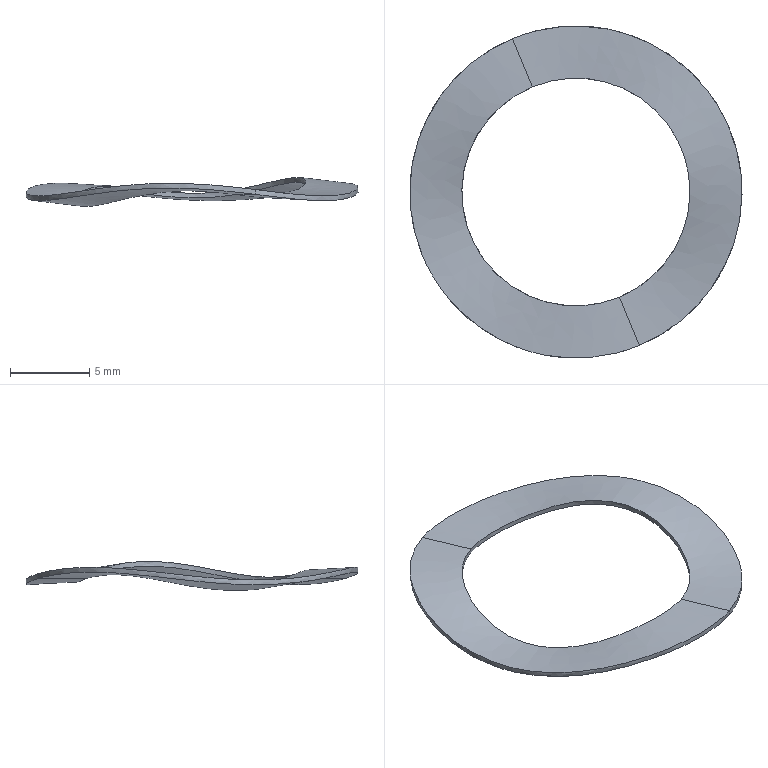Part | STEP file | MSBR-23_1_1_1_1 | 1 solid | 8 faces | box 21.008 x 21.003 x 1.851 mm | volume 55.347 mm3 | spline 4 | other 4
STEP:
#1=CARTESIAN_POINT('',(0.,0.,0.));
#2=DIRECTION('',(0.,0.,1.));
#3=DIRECTION('',(1.,0.,0.));
#4=AXIS2_PLACEMENT_3D('',#1,#2,#3);
#5=CARTESIAN_POINT('',(4.014,-9.702,86.503));
#6=VERTEX_POINT('',#5);
#7=CARTESIAN_POINT('',(2.75,-6.654,86.503));
#8=VERTEX_POINT('',#7);
#9=CARTESIAN_POINT('',(4.014,-9.702,86.503));
#10=DIRECTION('',(-0.383,0.9237,0.));
#11=VECTOR('',#10,3.3);
#12=LINE('',#9,#11);
#13=EDGE_CURVE('',#6,#8,#12,.T.);
#14=ORIENTED_EDGE('',*,*,#13,.F.);
#15=CARTESIAN_POINT('',(-4.03,9.696,86.503));
#16=VERTEX_POINT('',#15);
#17=CARTESIAN_POINT('',(-4.466,9.515,86.557));
#18=CARTESIAN_POINT('',(-5.302,9.099,86.663));
#19=CARTESIAN_POINT('',(-6.432,8.338,86.794));
#20=CARTESIAN_POINT('',(-7.446,7.45,86.881));
#21=CARTESIAN_POINT('',(-8.359,6.409,86.913));
#22=CARTESIAN_POINT('',(-9.107,5.296,86.884));
#23=CARTESIAN_POINT('',(-9.73,4.041,86.795));
#24=CARTESIAN_POINT('',(-10.168,2.76,86.665));
#25=CARTESIAN_POINT('',(-10.445,1.402,86.507));
#26=CARTESIAN_POINT('',(-10.54,-0.01496,86.345));
#27=CARTESIAN_POINT('',(-10.442,-1.421,86.209));
#28=CARTESIAN_POINT('',(-10.167,-2.768,86.122));
#29=CARTESIAN_POINT('',(-9.732,-4.039,86.093));
#30=CARTESIAN_POINT('',(-9.127,-5.267,86.124));
#31=CARTESIAN_POINT('',(-8.371,-6.401,86.211));
#32=CARTESIAN_POINT('',(-7.449,-7.456,86.346));
#33=CARTESIAN_POINT('',(-6.386,-8.382,86.507));
#34=CARTESIAN_POINT('',(-5.241,-9.14,86.663));
#35=CARTESIAN_POINT('',(-4.007,-9.746,86.796));
#36=CARTESIAN_POINT('',(-2.671,-10.19,86.884));
#37=CARTESIAN_POINT('',(-1.362,-10.445,86.913));
#38=CARTESIAN_POINT('',(0.02789,-10.533,86.88));
#39=CARTESIAN_POINT('',(1.365,-10.441,86.793));
#40=CARTESIAN_POINT('',(2.695,-10.18,86.663));
#41=CARTESIAN_POINT('',(3.579,-9.883,86.557));
#42=CARTESIAN_POINT('',(4.014,-9.702,86.503));
#43=B_SPLINE_CURVE_WITH_KNOTS('',3,(#15,#17,#18,#19,#20,#21,#22,#23,#24,#25,#26,#27,#28,#29,#30,#31,#32,#33,#34,#35,#36,#37,#38,#39,#40,#41,#42),.UNSPECIFIED.,.F.,.F.,(4,1,1,1,1,1,1,1,1,1,1,1,1,1,1,1,1,1,1,1,1,1,1,1,4),(0.,0.04167,0.08333,0.125,0.1667,0.2083,0.25,0.2917,0.3333,0.375,0.4167,0.4583,0.5,0.5417,0.5833,0.625,0.6667,0.7083,0.75,0.7917,0.8333,0.875,0.9167,0.9583,1.),.UNSPECIFIED.);
#44=EDGE_CURVE('',#16,#6,#43,.T.);
#45=ORIENTED_EDGE('',*,*,#44,.F.);
#46=CARTESIAN_POINT('',(-2.766,6.648,86.503));
#47=VERTEX_POINT('',#46);
#48=CARTESIAN_POINT('',(-2.766,6.648,86.503));
#49=DIRECTION('',(-0.383,0.9237,0.));
#50=VECTOR('',#49,3.3);
#51=LINE('',#48,#50);
#52=EDGE_CURVE('',#47,#16,#51,.T.);
#53=ORIENTED_EDGE('',*,*,#52,.F.);
#54=CARTESIAN_POINT('',(2.75,-6.654,86.503));
#55=CARTESIAN_POINT('',(2.431,-6.787,86.542));
#56=CARTESIAN_POINT('',(1.789,-6.999,86.618));
#57=CARTESIAN_POINT('',(0.8599,-7.171,86.699));
#58=CARTESIAN_POINT('',(-0.05536,-7.228,86.74));
#59=CARTESIAN_POINT('',(-1.07,-7.152,86.717));
#60=CARTESIAN_POINT('',(-1.966,-6.963,86.639));
#61=CARTESIAN_POINT('',(-2.947,-6.616,86.492));
#62=CARTESIAN_POINT('',(-3.833,-6.146,86.306));
#63=CARTESIAN_POINT('',(-4.631,-5.575,86.112));
#64=CARTESIAN_POINT('',(-5.371,-4.874,85.931));
#65=CARTESIAN_POINT('',(-6.022,-4.041,85.793));
#66=CARTESIAN_POINT('',(-6.494,-3.221,85.726));
#67=CARTESIAN_POINT('',(-6.856,-2.357,85.725));
#68=CARTESIAN_POINT('',(-7.111,-1.427,85.791));
#69=CARTESIAN_POINT('',(-7.241,-0.395,85.925));
#70=CARTESIAN_POINT('',(-7.222,0.593,86.099));
#71=CARTESIAN_POINT('',(-7.076,1.556,86.291));
#72=CARTESIAN_POINT('',(-6.782,2.546,86.484));
#73=CARTESIAN_POINT('',(-6.339,3.488,86.634));
#74=CARTESIAN_POINT('',(-5.834,4.274,86.715));
#75=CARTESIAN_POINT('',(-5.171,5.053,86.74));
#76=CARTESIAN_POINT('',(-4.467,5.677,86.7));
#77=CARTESIAN_POINT('',(-3.685,6.213,86.618));
#78=CARTESIAN_POINT('',(-3.083,6.516,86.542));
#79=CARTESIAN_POINT('',(-2.766,6.648,86.503));
#80=B_SPLINE_CURVE_WITH_KNOTS('',3,(#54,#55,#56,#57,#58,#59,#60,#61,#62,#63,#64,#65,#66,#67,#68,#69,#70,#71,#72,#73,#74,#75,#76,#77,#78,#79),.UNSPECIFIED.,.F.,.F.,(4,1,1,1,1,1,1,1,1,1,1,1,1,1,1,1,1,1,1,1,1,1,1,4),(0.,0.04348,0.08696,0.1304,0.1739,0.2174,0.2609,0.3043,0.3478,0.3913,0.4348,0.4783,0.5217,0.5652,0.6087,0.6522,0.6957,0.7391,0.7826,0.8261,0.8696,0.913,0.9565,1.),.UNSPECIFIED.);
#81=EDGE_CURVE('',#8,#47,#80,.T.);
#82=ORIENTED_EDGE('',*,*,#81,.F.);
#83=EDGE_LOOP('',(#14,#45,#53,#82));
#84=FACE_OUTER_BOUND('',#83,.F.);
#85=CARTESIAN_POINT('',(4.643,-9.491,86.428));
#86=CARTESIAN_POINT('',(4.14,-8.463,86.436));
#87=CARTESIAN_POINT('',(3.637,-7.436,86.444));
#88=CARTESIAN_POINT('',(3.135,-6.408,86.452));
#89=CARTESIAN_POINT('',(4.445,-9.588,86.452));
#90=CARTESIAN_POINT('',(3.963,-8.55,86.458));
#91=CARTESIAN_POINT('',(3.482,-7.512,86.463));
#92=CARTESIAN_POINT('',(3.,-6.474,86.469));
#93=CARTESIAN_POINT('',(3.805,-9.877,86.533));
#94=CARTESIAN_POINT('',(3.392,-8.808,86.529));
#95=CARTESIAN_POINT('',(2.979,-7.739,86.526));
#96=CARTESIAN_POINT('',(2.566,-6.67,86.523));
#97=CARTESIAN_POINT('',(2.682,-10.255,86.668));
#98=CARTESIAN_POINT('',(2.388,-9.146,86.65));
#99=CARTESIAN_POINT('',(2.095,-8.037,86.632));
#100=CARTESIAN_POINT('',(1.802,-6.927,86.615));
#101=CARTESIAN_POINT('',(1.261,-10.526,86.805));
#102=CARTESIAN_POINT('',(1.12,-9.387,86.77));
#103=CARTESIAN_POINT('',(0.9801,-8.249,86.735));
#104=CARTESIAN_POINT('',(0.8399,-7.111,86.7));
#105=CARTESIAN_POINT('',(-0.1842,-10.601,86.893));
#106=CARTESIAN_POINT('',(-0.1673,-9.454,86.841));
#107=CARTESIAN_POINT('',(-0.1505,-8.308,86.789));
#108=CARTESIAN_POINT('',(-0.1336,-7.161,86.738));
#109=CARTESIAN_POINT('',(-1.626,-10.478,86.917));
#110=CARTESIAN_POINT('',(-1.45,-9.345,86.849));
#111=CARTESIAN_POINT('',(-1.275,-8.213,86.781));
#112=CARTESIAN_POINT('',(-1.1,-7.081,86.713));
#113=CARTESIAN_POINT('',(-3.037,-10.16,86.873));
#114=CARTESIAN_POINT('',(-2.706,-9.064,86.79));
#115=CARTESIAN_POINT('',(-2.374,-7.968,86.707));
#116=CARTESIAN_POINT('',(-2.043,-6.872,86.624));
#117=CARTESIAN_POINT('',(-4.392,-9.652,86.768));
#118=CARTESIAN_POINT('',(-3.911,-8.615,86.672));
#119=CARTESIAN_POINT('',(-3.43,-7.577,86.576));
#120=CARTESIAN_POINT('',(-2.949,-6.539,86.479));
#121=CARTESIAN_POINT('',(-5.665,-8.965,86.62));
#122=CARTESIAN_POINT('',(-5.045,-8.006,86.513));
#123=CARTESIAN_POINT('',(-4.425,-7.046,86.405));
#124=CARTESIAN_POINT('',(-3.805,-6.086,86.298));
#125=CARTESIAN_POINT('',(-6.833,-8.111,86.454));
#126=CARTESIAN_POINT('',(-6.087,-7.247,86.337));
#127=CARTESIAN_POINT('',(-5.342,-6.382,86.22));
#128=CARTESIAN_POINT('',(-4.596,-5.518,86.104));
#129=CARTESIAN_POINT('',(-7.873,-7.106,86.296));
#130=CARTESIAN_POINT('',(-7.018,-6.351,86.173));
#131=CARTESIAN_POINT('',(-6.164,-5.596,86.05));
#132=CARTESIAN_POINT('',(-5.309,-4.841,85.926));
#133=CARTESIAN_POINT('',(-8.767,-5.969,86.174));
#134=CARTESIAN_POINT('',(-7.82,-5.335,86.046));
#135=CARTESIAN_POINT('',(-6.873,-4.7,85.919));
#136=CARTESIAN_POINT('',(-5.926,-4.065,85.791));
#137=CARTESIAN_POINT('',(-9.498,-4.721,86.108));
#138=CARTESIAN_POINT('',(-8.476,-4.217,85.978));
#139=CARTESIAN_POINT('',(-7.454,-3.712,85.848));
#140=CARTESIAN_POINT('',(-6.432,-3.207,85.718));
#141=CARTESIAN_POINT('',(-10.052,-3.385,86.108));
#142=CARTESIAN_POINT('',(-8.973,-3.019,85.978));
#143=CARTESIAN_POINT('',(-7.893,-2.652,85.848));
#144=CARTESIAN_POINT('',(-6.814,-2.285,85.718));
#145=CARTESIAN_POINT('',(-10.419,-1.987,86.174));
#146=CARTESIAN_POINT('',(-9.3,-1.765,86.046));
#147=CARTESIAN_POINT('',(-8.182,-1.543,85.919));
#148=CARTESIAN_POINT('',(-7.064,-1.321,85.791));
#149=CARTESIAN_POINT('',(-10.592,-0.5507,86.296));
#150=CARTESIAN_POINT('',(-9.453,-0.4793,86.173));
#151=CARTESIAN_POINT('',(-8.315,-0.408,86.05));
#152=CARTESIAN_POINT('',(-7.176,-0.3367,85.926));
#153=CARTESIAN_POINT('',(-10.568,0.8956,86.454));
#154=CARTESIAN_POINT('',(-9.429,0.8123,86.337));
#155=CARTESIAN_POINT('',(-8.291,0.7291,86.22));
#156=CARTESIAN_POINT('',(-7.152,0.6458,86.104));
#157=CARTESIAN_POINT('',(-10.347,2.325,86.62));
#158=CARTESIAN_POINT('',(-9.23,2.086,86.513));
#159=CARTESIAN_POINT('',(-8.113,1.847,86.405));
#160=CARTESIAN_POINT('',(-6.995,1.608,86.298));
#161=CARTESIAN_POINT('',(-9.934,3.712,86.768));
#162=CARTESIAN_POINT('',(-8.86,3.319,86.672));
#163=CARTESIAN_POINT('',(-7.786,2.926,86.576));
#164=CARTESIAN_POINT('',(-6.711,2.534,86.479));
#165=CARTESIAN_POINT('',(-9.336,5.029,86.873));
#166=CARTESIAN_POINT('',(-8.326,4.489,86.79));
#167=CARTESIAN_POINT('',(-7.316,3.95,86.707));
#168=CARTESIAN_POINT('',(-6.307,3.41,86.624));
#169=CARTESIAN_POINT('',(-8.563,6.253,86.917));
#170=CARTESIAN_POINT('',(-7.638,5.577,86.849));
#171=CARTESIAN_POINT('',(-6.713,4.901,86.781));
#172=CARTESIAN_POINT('',(-5.788,4.225,86.713));
#173=CARTESIAN_POINT('',(-7.632,7.359,86.893));
#174=CARTESIAN_POINT('',(-6.809,6.561,86.841));
#175=CARTESIAN_POINT('',(-5.985,5.763,86.789));
#176=CARTESIAN_POINT('',(-5.162,4.965,86.738));
#177=CARTESIAN_POINT('',(-6.558,8.329,86.805));
#178=CARTESIAN_POINT('',(-5.852,7.425,86.77));
#179=CARTESIAN_POINT('',(-5.145,6.522,86.735));
#180=CARTESIAN_POINT('',(-4.438,5.618,86.7));
#181=CARTESIAN_POINT('',(-5.363,9.143,86.668));
#182=CARTESIAN_POINT('',(-4.785,8.152,86.65));
#183=CARTESIAN_POINT('',(-4.207,7.161,86.632));
#184=CARTESIAN_POINT('',(-3.629,6.17,86.615));
#185=CARTESIAN_POINT('',(-4.301,9.671,86.533));
#186=CARTESIAN_POINT('',(-3.837,8.624,86.529));
#187=CARTESIAN_POINT('',(-3.372,7.576,86.526));
#188=CARTESIAN_POINT('',(-2.908,6.528,86.523));
#189=CARTESIAN_POINT('',(-3.645,9.92,86.452));
#190=CARTESIAN_POINT('',(-3.25,8.845,86.458));
#191=CARTESIAN_POINT('',(-2.856,7.771,86.463));
#192=CARTESIAN_POINT('',(-2.462,6.697,86.469));
#193=CARTESIAN_POINT('',(-3.436,9.991,86.428));
#194=CARTESIAN_POINT('',(-3.064,8.909,86.436));
#195=CARTESIAN_POINT('',(-2.692,7.828,86.444));
#196=CARTESIAN_POINT('',(-2.32,6.746,86.452));
#197=B_SPLINE_SURFACE_WITH_KNOTS('',3,3,((#85,#86,#87,#88),(#89,#90,#91,#92),(#93,#94,#95,#96),(#97,#98,#99,#100),(#101,#102,#103,#104),(#105,#106,#107,#108),(#109,#110,#111,#112),(#113,#114,#115,#116),(#117,#118,#119,#120),(#121,#122,#123,#124),(#125,#126,#127,#128),(#129,#130,#131,#132),(#133,#134,#135,#136),(#137,#138,#139,#140),(#141,#142,#143,#144),(#145,#146,#147,#148),(#149,#150,#151,#152),(#153,#154,#155,#156),(#157,#158,#159,#160),(#161,#162,#163,#164),(#165,#166,#167,#168),(#169,#170,#171,#172),(#173,#174,#175,#176),(#177,#178,#179,#180),(#181,#182,#183,#184),(#185,#186,#187,#188),(#189,#190,#191,#192),(#193,#194,#195,#196)),.UNSPECIFIED.,.F.,.F.,.F.,(4,1,1,1,1,1,1,1,1,1,1,1,1,1,1,1,1,1,1,1,1,1,1,1,1,4),(4,4),(-0.01993,0.,0.04348,0.08696,0.1304,0.1739,0.2174,0.2609,0.3043,0.3478,0.3913,0.4348,0.4783,0.5217,0.5652,0.6087,0.6522,0.6957,0.7391,0.7826,0.8261,0.8696,0.913,0.9565,1.,1.02),(-0.000000563,1.),.UNSPECIFIED.);
#198=ADVANCED_FACE('',(#84),#197,.F.);
#199=CARTESIAN_POINT('',(-2.766,6.648,86.503));
#200=CARTESIAN_POINT('',(-2.446,6.78,86.463));
#201=CARTESIAN_POINT('',(-1.804,6.992,86.388));
#202=CARTESIAN_POINT('',(-0.875,7.165,86.306));
#203=CARTESIAN_POINT('',(0.04021,7.222,86.266));
#204=CARTESIAN_POINT('',(1.055,7.145,86.289));
#205=CARTESIAN_POINT('',(1.951,6.956,86.367));
#206=CARTESIAN_POINT('',(2.932,6.61,86.514));
#207=CARTESIAN_POINT('',(3.818,6.14,86.699));
#208=CARTESIAN_POINT('',(4.616,5.569,86.893));
#209=CARTESIAN_POINT('',(5.356,4.868,87.075));
#210=CARTESIAN_POINT('',(6.007,4.035,87.213));
#211=CARTESIAN_POINT('',(6.479,3.215,87.279));
#212=CARTESIAN_POINT('',(6.841,2.351,87.28));
#213=CARTESIAN_POINT('',(7.096,1.421,87.214));
#214=CARTESIAN_POINT('',(7.226,0.3888,87.08));
#215=CARTESIAN_POINT('',(7.207,-0.5992,86.907));
#216=CARTESIAN_POINT('',(7.061,-1.562,86.714));
#217=CARTESIAN_POINT('',(6.767,-2.552,86.522));
#218=CARTESIAN_POINT('',(6.324,-3.495,86.372));
#219=CARTESIAN_POINT('',(5.819,-4.28,86.29));
#220=CARTESIAN_POINT('',(5.155,-5.059,86.265));
#221=CARTESIAN_POINT('',(4.452,-5.683,86.306));
#222=CARTESIAN_POINT('',(3.67,-6.219,86.388));
#223=CARTESIAN_POINT('',(3.068,-6.522,86.464));
#224=CARTESIAN_POINT('',(2.75,-6.654,86.503));
#225=B_SPLINE_CURVE_WITH_KNOTS('',3,(#199,#200,#201,#202,#203,#204,#205,#206,#207,#208,#209,#210,#211,#212,#213,#214,#215,#216,#217,#218,#219,#220,#221,#222,#223,#224),.UNSPECIFIED.,.F.,.F.,(4,1,1,1,1,1,1,1,1,1,1,1,1,1,1,1,1,1,1,1,1,1,1,4),(0.,0.04348,0.08696,0.1304,0.1739,0.2174,0.2609,0.3043,0.3478,0.3913,0.4348,0.4783,0.5217,0.5652,0.6087,0.6522,0.6957,0.7391,0.7826,0.8261,0.8696,0.913,0.9565,1.),.UNSPECIFIED.);
#226=EDGE_CURVE('',#47,#8,#225,.T.);
#227=ORIENTED_EDGE('',*,*,#226,.F.);
#228=ORIENTED_EDGE('',*,*,#52,.T.);
#229=CARTESIAN_POINT('',(4.014,-9.702,86.503));
#230=CARTESIAN_POINT('',(4.448,-9.523,86.449));
#231=CARTESIAN_POINT('',(5.28,-9.109,86.345));
#232=CARTESIAN_POINT('',(6.406,-8.352,86.214));
#233=CARTESIAN_POINT('',(7.42,-7.467,86.124));
#234=CARTESIAN_POINT('',(8.335,-6.426,86.096));
#235=CARTESIAN_POINT('',(9.083,-5.317,86.124));
#236=CARTESIAN_POINT('',(9.712,-4.057,86.21));
#237=CARTESIAN_POINT('',(10.15,-2.776,86.34));
#238=CARTESIAN_POINT('',(10.428,-1.421,86.498));
#239=CARTESIAN_POINT('',(10.525,-0.00639,86.659));
#240=CARTESIAN_POINT('',(10.428,1.411,86.794));
#241=CARTESIAN_POINT('',(10.151,2.764,86.882));
#242=CARTESIAN_POINT('',(9.719,4.027,86.913));
#243=CARTESIAN_POINT('',(9.114,5.257,86.881));
#244=CARTESIAN_POINT('',(8.36,6.39,86.793));
#245=CARTESIAN_POINT('',(7.434,7.449,86.66));
#246=CARTESIAN_POINT('',(6.371,8.376,86.499));
#247=CARTESIAN_POINT('',(5.227,9.133,86.343));
#248=CARTESIAN_POINT('',(3.994,9.738,86.21));
#249=CARTESIAN_POINT('',(2.653,10.185,86.123));
#250=CARTESIAN_POINT('',(1.338,10.44,86.095));
#251=CARTESIAN_POINT('',(-0.0515,10.527,86.125));
#252=CARTESIAN_POINT('',(-1.392,10.434,86.215));
#253=CARTESIAN_POINT('',(-2.716,10.172,86.345));
#254=CARTESIAN_POINT('',(-3.596,9.876,86.449));
#255=CARTESIAN_POINT('',(-4.03,9.696,86.503));
#256=B_SPLINE_CURVE_WITH_KNOTS('',3,(#229,#230,#231,#232,#233,#234,#235,#236,#237,#238,#239,#240,#241,#242,#243,#244,#245,#246,#247,#248,#249,#250,#251,#252,#253,#254,#255),.UNSPECIFIED.,.F.,.F.,(4,1,1,1,1,1,1,1,1,1,1,1,1,1,1,1,1,1,1,1,1,1,1,1,4),(0.,0.04167,0.08333,0.125,0.1667,0.2083,0.25,0.2917,0.3333,0.375,0.4167,0.4583,0.5,0.5417,0.5833,0.625,0.6667,0.7083,0.75,0.7917,0.8333,0.875,0.9167,0.9583,1.),.UNSPECIFIED.);
#257=EDGE_CURVE('',#6,#16,#256,.T.);
#258=ORIENTED_EDGE('',*,*,#257,.F.);
#259=ORIENTED_EDGE('',*,*,#13,.T.);
#260=EDGE_LOOP('',(#227,#228,#258,#259));
#261=FACE_OUTER_BOUND('',#260,.F.);
#262=CARTESIAN_POINT('',(-4.658,9.485,86.578));
#263=CARTESIAN_POINT('',(-4.155,8.457,86.57));
#264=CARTESIAN_POINT('',(-3.652,7.429,86.562));
#265=CARTESIAN_POINT('',(-3.15,6.402,86.554));
#266=CARTESIAN_POINT('',(-4.46,9.582,86.553));
#267=CARTESIAN_POINT('',(-3.978,8.544,86.548));
#268=CARTESIAN_POINT('',(-3.497,7.506,86.542));
#269=CARTESIAN_POINT('',(-3.015,6.468,86.537));
#270=CARTESIAN_POINT('',(-3.82,9.871,86.473));
#271=CARTESIAN_POINT('',(-3.407,8.802,86.476));
#272=CARTESIAN_POINT('',(-2.994,7.733,86.479));
#273=CARTESIAN_POINT('',(-2.581,6.664,86.483));
#274=CARTESIAN_POINT('',(-2.697,10.249,86.338));
#275=CARTESIAN_POINT('',(-2.404,9.14,86.356));
#276=CARTESIAN_POINT('',(-2.111,8.03,86.373));
#277=CARTESIAN_POINT('',(-1.817,6.921,86.391));
#278=CARTESIAN_POINT('',(-1.276,10.52,86.2));
#279=CARTESIAN_POINT('',(-1.135,9.381,86.235));
#280=CARTESIAN_POINT('',(-0.9952,8.243,86.27));
#281=CARTESIAN_POINT('',(-0.855,7.104,86.305));
#282=CARTESIAN_POINT('',(0.1691,10.594,86.112));
#283=CARTESIAN_POINT('',(0.1522,9.448,86.164));
#284=CARTESIAN_POINT('',(0.1354,8.301,86.216));
#285=CARTESIAN_POINT('',(0.1185,7.155,86.268));
#286=CARTESIAN_POINT('',(1.611,10.471,86.088));
#287=CARTESIAN_POINT('',(1.435,9.339,86.157));
#288=CARTESIAN_POINT('',(1.26,8.207,86.225));
#289=CARTESIAN_POINT('',(1.085,7.075,86.293));
#290=CARTESIAN_POINT('',(3.022,10.153,86.133));
#291=CARTESIAN_POINT('',(2.691,9.058,86.216));
#292=CARTESIAN_POINT('',(2.359,7.962,86.299));
#293=CARTESIAN_POINT('',(2.028,6.866,86.382));
#294=CARTESIAN_POINT('',(4.377,9.646,86.238));
#295=CARTESIAN_POINT('',(3.896,8.608,86.334));
#296=CARTESIAN_POINT('',(3.415,7.571,86.43));
#297=CARTESIAN_POINT('',(2.934,6.533,86.526));
#298=CARTESIAN_POINT('',(5.65,8.959,86.386));
#299=CARTESIAN_POINT('',(5.03,7.999,86.493));
#300=CARTESIAN_POINT('',(4.41,7.04,86.601));
#301=CARTESIAN_POINT('',(3.79,6.08,86.708));
#302=CARTESIAN_POINT('',(6.818,8.105,86.552));
#303=CARTESIAN_POINT('',(6.072,7.241,86.669));
#304=CARTESIAN_POINT('',(5.327,6.376,86.785));
#305=CARTESIAN_POINT('',(4.581,5.511,86.902));
#306=CARTESIAN_POINT('',(7.858,7.1,86.709));
#307=CARTESIAN_POINT('',(7.003,6.345,86.833));
#308=CARTESIAN_POINT('',(6.148,5.59,86.956));
#309=CARTESIAN_POINT('',(5.294,4.834,87.079));
#310=CARTESIAN_POINT('',(8.752,5.963,86.832));
#311=CARTESIAN_POINT('',(7.805,5.328,86.959));
#312=CARTESIAN_POINT('',(6.858,4.694,87.087));
#313=CARTESIAN_POINT('',(5.91,4.059,87.215));
#314=CARTESIAN_POINT('',(9.483,4.715,86.898));
#315=CARTESIAN_POINT('',(8.461,4.21,87.028));
#316=CARTESIAN_POINT('',(7.439,3.706,87.158));
#317=CARTESIAN_POINT('',(6.417,3.201,87.288));
#318=CARTESIAN_POINT('',(10.037,3.379,86.898));
#319=CARTESIAN_POINT('',(8.957,3.012,87.028));
#320=CARTESIAN_POINT('',(7.878,2.646,87.158));
#321=CARTESIAN_POINT('',(6.799,2.279,87.288));
#322=CARTESIAN_POINT('',(10.404,1.98,86.832));
#323=CARTESIAN_POINT('',(9.285,1.758,86.959));
#324=CARTESIAN_POINT('',(8.167,1.537,87.087));
#325=CARTESIAN_POINT('',(7.049,1.315,87.215));
#326=CARTESIAN_POINT('',(10.577,0.5444,86.709));
#327=CARTESIAN_POINT('',(9.438,0.4731,86.833));
#328=CARTESIAN_POINT('',(8.3,0.4017,86.956));
#329=CARTESIAN_POINT('',(7.161,0.3304,87.079));
#330=CARTESIAN_POINT('',(10.553,-0.9019,86.552));
#331=CARTESIAN_POINT('',(9.414,-0.8186,86.669));
#332=CARTESIAN_POINT('',(8.276,-0.7353,86.785));
#333=CARTESIAN_POINT('',(7.137,-0.6521,86.902));
#334=CARTESIAN_POINT('',(10.332,-2.332,86.386));
#335=CARTESIAN_POINT('',(9.215,-2.092,86.493));
#336=CARTESIAN_POINT('',(8.098,-1.853,86.601));
#337=CARTESIAN_POINT('',(6.98,-1.614,86.708));
#338=CARTESIAN_POINT('',(9.919,-3.718,86.238));
#339=CARTESIAN_POINT('',(8.845,-3.325,86.334));
#340=CARTESIAN_POINT('',(7.77,-2.933,86.43));
#341=CARTESIAN_POINT('',(6.696,-2.54,86.526));
#342=CARTESIAN_POINT('',(9.32,-5.035,86.133));
#343=CARTESIAN_POINT('',(8.311,-4.496,86.216));
#344=CARTESIAN_POINT('',(7.301,-3.956,86.299));
#345=CARTESIAN_POINT('',(6.292,-3.416,86.382));
#346=CARTESIAN_POINT('',(8.548,-6.259,86.088));
#347=CARTESIAN_POINT('',(7.623,-5.583,86.157));
#348=CARTESIAN_POINT('',(6.698,-4.907,86.225));
#349=CARTESIAN_POINT('',(5.773,-4.231,86.293));
#350=CARTESIAN_POINT('',(7.617,-7.366,86.112));
#351=CARTESIAN_POINT('',(6.793,-6.568,86.164));
#352=CARTESIAN_POINT('',(5.97,-5.77,86.216));
#353=CARTESIAN_POINT('',(5.147,-4.972,86.268));
#354=CARTESIAN_POINT('',(6.543,-8.335,86.2));
#355=CARTESIAN_POINT('',(5.836,-7.432,86.235));
#356=CARTESIAN_POINT('',(5.13,-6.528,86.27));
#357=CARTESIAN_POINT('',(4.423,-5.625,86.305));
#358=CARTESIAN_POINT('',(5.348,-9.15,86.338));
#359=CARTESIAN_POINT('',(4.77,-8.158,86.356));
#360=CARTESIAN_POINT('',(4.192,-7.167,86.373));
#361=CARTESIAN_POINT('',(3.614,-6.176,86.391));
#362=CARTESIAN_POINT('',(4.286,-9.677,86.473));
#363=CARTESIAN_POINT('',(3.822,-8.63,86.476));
#364=CARTESIAN_POINT('',(3.357,-7.582,86.479));
#365=CARTESIAN_POINT('',(2.893,-6.535,86.483));
#366=CARTESIAN_POINT('',(3.63,-9.926,86.553));
#367=CARTESIAN_POINT('',(3.235,-8.852,86.548));
#368=CARTESIAN_POINT('',(2.841,-7.778,86.542));
#369=CARTESIAN_POINT('',(2.447,-6.703,86.537));
#370=CARTESIAN_POINT('',(3.421,-9.997,86.578));
#371=CARTESIAN_POINT('',(3.049,-8.916,86.57));
#372=CARTESIAN_POINT('',(2.677,-7.834,86.562));
#373=CARTESIAN_POINT('',(2.305,-6.752,86.554));
#374=B_SPLINE_SURFACE_WITH_KNOTS('',3,3,((#262,#263,#264,#265),(#266,#267,#268,#269),(#270,#271,#272,#273),(#274,#275,#276,#277),(#278,#279,#280,#281),(#282,#283,#284,#285),(#286,#287,#288,#289),(#290,#291,#292,#293),(#294,#295,#296,#297),(#298,#299,#300,#301),(#302,#303,#304,#305),(#306,#307,#308,#309),(#310,#311,#312,#313),(#314,#315,#316,#317),(#318,#319,#320,#321),(#322,#323,#324,#325),(#326,#327,#328,#329),(#330,#331,#332,#333),(#334,#335,#336,#337),(#338,#339,#340,#341),(#342,#343,#344,#345),(#346,#347,#348,#349),(#350,#351,#352,#353),(#354,#355,#356,#357),(#358,#359,#360,#361),(#362,#363,#364,#365),(#366,#367,#368,#369),(#370,#371,#372,#373)),.UNSPECIFIED.,.F.,.F.,.F.,(4,1,1,1,1,1,1,1,1,1,1,1,1,1,1,1,1,1,1,1,1,1,1,1,1,4),(4,4),(-0.01993,0.,0.04348,0.08696,0.1304,0.1739,0.2174,0.2609,0.3043,0.3478,0.3913,0.4348,0.4783,0.5217,0.5652,0.6087,0.6522,0.6957,0.7391,0.7826,0.8261,0.8696,0.913,0.9565,1.,1.02),(-0.000000504,1.),.UNSPECIFIED.);
#375=ADVANCED_FACE('',(#261),#374,.F.);
#376=CARTESIAN_POINT('',(2.758,-6.651,86.2));
#377=VERTEX_POINT('',#376);
#378=CARTESIAN_POINT('',(2.758,-6.651,86.2));
#379=DIRECTION('',(-0.02492,-0.01034,0.9996));
#380=VECTOR('',#379,0.3029);
#381=LINE('',#378,#380);
#382=EDGE_CURVE('',#377,#8,#381,.T.);
#383=ORIENTED_EDGE('',*,*,#382,.F.);
#384=CARTESIAN_POINT('',(-2.758,6.651,86.2));
#385=VERTEX_POINT('',#384);
#386=CARTESIAN_POINT('',(2.758,-6.651,86.2));
#387=CARTESIAN_POINT('',(3.078,-6.518,86.16));
#388=CARTESIAN_POINT('',(3.681,-6.214,86.085));
#389=CARTESIAN_POINT('',(4.458,-5.68,86.003));
#390=CARTESIAN_POINT('',(5.147,-5.071,85.963));
#391=CARTESIAN_POINT('',(5.808,-4.3,85.986));
#392=CARTESIAN_POINT('',(6.308,-3.532,86.064));
#393=CARTESIAN_POINT('',(6.756,-2.593,86.211));
#394=CARTESIAN_POINT('',(7.05,-1.634,86.397));
#395=CARTESIAN_POINT('',(7.209,-0.6651,86.591));
#396=CARTESIAN_POINT('',(7.237,0.3536,86.772));
#397=CARTESIAN_POINT('',(7.107,1.402,86.909));
#398=CARTESIAN_POINT('',(6.86,2.318,86.976));
#399=CARTESIAN_POINT('',(6.504,3.184,86.978));
#400=CARTESIAN_POINT('',(6.027,4.02,86.912));
#401=CARTESIAN_POINT('',(5.388,4.841,86.778));
#402=CARTESIAN_POINT('',(4.675,5.527,86.604));
#403=CARTESIAN_POINT('',(3.89,6.103,86.412));
#404=CARTESIAN_POINT('',(2.983,6.594,86.219));
#405=CARTESIAN_POINT('',(2.004,6.947,86.069));
#406=CARTESIAN_POINT('',(1.091,7.145,85.987));
#407=CARTESIAN_POINT('',(0.06972,7.226,85.962));
#408=CARTESIAN_POINT('',(-0.8655,7.169,86.003));
#409=CARTESIAN_POINT('',(-1.799,6.995,86.085));
#410=CARTESIAN_POINT('',(-2.44,6.783,86.161));
#411=B_SPLINE_CURVE_WITH_KNOTS('',3,(#386,#387,#388,#389,#390,#391,#392,#393,#394,#395,#396,#397,#398,#399,#400,#401,#402,#403,#404,#405,#406,#407,#408,#409,#410,#384),.UNSPECIFIED.,.F.,.F.,(4,1,1,1,1,1,1,1,1,1,1,1,1,1,1,1,1,1,1,1,1,1,1,4),(0.,0.04348,0.08696,0.1304,0.1739,0.2174,0.2609,0.3043,0.3478,0.3913,0.4348,0.4783,0.5217,0.5652,0.6087,0.6522,0.6957,0.7391,0.7826,0.8261,0.8696,0.913,0.9565,1.),.UNSPECIFIED.);
#412=EDGE_CURVE('',#377,#385,#411,.T.);
#413=ORIENTED_EDGE('',*,*,#412,.T.);
#414=CARTESIAN_POINT('',(-2.766,6.648,86.503));
#415=DIRECTION('',(0.02492,0.01034,-0.9996));
#416=VECTOR('',#415,0.3029);
#417=LINE('',#414,#416);
#418=EDGE_CURVE('',#47,#385,#417,.T.);
#419=ORIENTED_EDGE('',*,*,#418,.F.);
#420=ORIENTED_EDGE('',*,*,#226,.T.);
#421=EDGE_LOOP('',(#383,#413,#419,#420));
#422=FACE_OUTER_BOUND('',#421,.F.);
#423=CARTESIAN_POINT('',(-3.162,6.468,85.839));
#424=CARTESIAN_POINT('',(-3.027,6.534,85.844));
#425=CARTESIAN_POINT('',(-2.458,6.791,85.86));
#426=CARTESIAN_POINT('',(-1.632,7.042,85.884));
#427=CARTESIAN_POINT('',(-0.6995,7.18,85.908));
#428=CARTESIAN_POINT('',(0.2397,7.227,85.932));
#429=CARTESIAN_POINT('',(1.175,7.137,85.955));
#430=CARTESIAN_POINT('',(2.083,6.915,85.975));
#431=CARTESIAN_POINT('',(2.967,6.607,85.994));
#432=CARTESIAN_POINT('',(4.011,6.064,86.014));
#433=CARTESIAN_POINT('',(5.124,5.175,86.033));
#434=CARTESIAN_POINT('',(5.896,4.255,86.042));
#435=CARTESIAN_POINT('',(6.395,3.433,86.046));
#436=CARTESIAN_POINT('',(6.705,2.78,86.047));
#437=CARTESIAN_POINT('',(6.947,2.1,86.046));
#438=CARTESIAN_POINT('',(7.177,1.166,86.042));
#439=CARTESIAN_POINT('',(7.283,-0.03002,86.033));
#440=CARTESIAN_POINT('',(7.125,-1.447,86.014));
#441=CARTESIAN_POINT('',(6.772,-2.569,85.994));
#442=CARTESIAN_POINT('',(6.365,-3.411,85.975));
#443=CARTESIAN_POINT('',(5.881,-4.211,85.954));
#444=CARTESIAN_POINT('',(5.283,-4.936,85.932));
#445=CARTESIAN_POINT('',(4.587,-5.568,85.908));
#446=CARTESIAN_POINT('',(3.83,-6.13,85.884));
#447=CARTESIAN_POINT('',(3.136,-6.502,85.862));
#448=CARTESIAN_POINT('',(2.627,-6.704,85.848));
#449=CARTESIAN_POINT('',(2.556,-6.731,85.846));
#450=B_SPLINE_CURVE_WITH_KNOTS('',3,(#423,#424,#425,#426,#427,#428,#429,#430,#431,#432,#433,#434,#435,#436,#437,#438,#439,#440,#441,#442,#443,#444,#445,#446,#447,#448,#449),.UNSPECIFIED.,.F.,.F.,(4,1,1,1,1,1,1,1,1,1,1,1,1,1,1,1,1,1,1,1,1,1,1,1,4),(0.,0.01941,0.08009,0.1104,0.1408,0.2015,0.2318,0.2621,0.3228,0.3835,0.4442,0.4745,0.5049,0.5352,0.5655,0.6262,0.6869,0.7476,0.7779,0.8083,0.8689,0.8993,0.9296,0.9903,1.),.UNSPECIFIED.);
#451=DIRECTION('',(-0.02492,-0.01034,0.9996));
#452=VECTOR('',#451,1.);
#453=SURFACE_OF_LINEAR_EXTRUSION('',#450,#452);
#454=ADVANCED_FACE('',(#422),#453,.T.);
#455=ORIENTED_EDGE('',*,*,#81,.T.);
#456=ORIENTED_EDGE('',*,*,#418,.T.);
#457=CARTESIAN_POINT('',(-2.758,6.651,86.2));
#458=CARTESIAN_POINT('',(-3.078,6.518,86.24));
#459=CARTESIAN_POINT('',(-3.681,6.214,86.315));
#460=CARTESIAN_POINT('',(-4.458,5.68,86.397));
#461=CARTESIAN_POINT('',(-5.147,5.071,86.437));
#462=CARTESIAN_POINT('',(-5.808,4.3,86.414));
#463=CARTESIAN_POINT('',(-6.308,3.532,86.336));
#464=CARTESIAN_POINT('',(-6.756,2.593,86.189));
#465=CARTESIAN_POINT('',(-7.05,1.634,86.003));
#466=CARTESIAN_POINT('',(-7.209,0.6651,85.809));
#467=CARTESIAN_POINT('',(-7.237,-0.3536,85.628));
#468=CARTESIAN_POINT('',(-7.107,-1.402,85.491));
#469=CARTESIAN_POINT('',(-6.86,-2.318,85.424));
#470=CARTESIAN_POINT('',(-6.504,-3.184,85.422));
#471=CARTESIAN_POINT('',(-6.027,-4.02,85.488));
#472=CARTESIAN_POINT('',(-5.388,-4.841,85.622));
#473=CARTESIAN_POINT('',(-4.675,-5.527,85.796));
#474=CARTESIAN_POINT('',(-3.89,-6.103,85.988));
#475=CARTESIAN_POINT('',(-2.983,-6.594,86.181));
#476=CARTESIAN_POINT('',(-2.004,-6.947,86.331));
#477=CARTESIAN_POINT('',(-1.091,-7.145,86.413));
#478=CARTESIAN_POINT('',(-0.06976,-7.226,86.438));
#479=CARTESIAN_POINT('',(0.8655,-7.169,86.397));
#480=CARTESIAN_POINT('',(1.799,-6.995,86.315));
#481=CARTESIAN_POINT('',(2.44,-6.783,86.239));
#482=CARTESIAN_POINT('',(2.758,-6.651,86.2));
#483=B_SPLINE_CURVE_WITH_KNOTS('',3,(#457,#458,#459,#460,#461,#462,#463,#464,#465,#466,#467,#468,#469,#470,#471,#472,#473,#474,#475,#476,#477,#478,#479,#480,#481,#482),.UNSPECIFIED.,.F.,.F.,(4,1,1,1,1,1,1,1,1,1,1,1,1,1,1,1,1,1,1,1,1,1,1,4),(0.,0.04348,0.08696,0.1304,0.1739,0.2174,0.2609,0.3043,0.3478,0.3913,0.4348,0.4783,0.5217,0.5652,0.6087,0.6522,0.6957,0.7391,0.7826,0.8261,0.8696,0.913,0.9565,1.),.UNSPECIFIED.);
#484=EDGE_CURVE('',#385,#377,#483,.T.);
#485=ORIENTED_EDGE('',*,*,#484,.T.);
#486=ORIENTED_EDGE('',*,*,#382,.T.);
#487=EDGE_LOOP('',(#455,#456,#485,#486));
#488=FACE_OUTER_BOUND('',#487,.F.);
#489=CARTESIAN_POINT('',(2.981,-6.554,85.591));
#490=CARTESIAN_POINT('',(2.912,-6.586,85.589));
#491=CARTESIAN_POINT('',(2.41,-6.803,85.574));
#492=CARTESIAN_POINT('',(1.656,-7.032,85.553));
#493=CARTESIAN_POINT('',(0.7235,-7.17,85.528));
#494=CARTESIAN_POINT('',(-0.2157,-7.217,85.504));
#495=CARTESIAN_POINT('',(-1.151,-7.127,85.482));
#496=CARTESIAN_POINT('',(-2.059,-6.905,85.462));
#497=CARTESIAN_POINT('',(-2.943,-6.597,85.443));
#498=CARTESIAN_POINT('',(-3.987,-6.055,85.422));
#499=CARTESIAN_POINT('',(-5.1,-5.165,85.404));
#500=CARTESIAN_POINT('',(-5.872,-4.245,85.394));
#501=CARTESIAN_POINT('',(-6.371,-3.423,85.39));
#502=CARTESIAN_POINT('',(-6.681,-2.77,85.389));
#503=CARTESIAN_POINT('',(-6.923,-2.09,85.39));
#504=CARTESIAN_POINT('',(-7.153,-1.156,85.394));
#505=CARTESIAN_POINT('',(-7.259,0.03999,85.404));
#506=CARTESIAN_POINT('',(-7.101,1.457,85.423));
#507=CARTESIAN_POINT('',(-6.748,2.579,85.443));
#508=CARTESIAN_POINT('',(-6.341,3.421,85.462));
#509=CARTESIAN_POINT('',(-5.857,4.221,85.482));
#510=CARTESIAN_POINT('',(-5.259,4.946,85.505));
#511=CARTESIAN_POINT('',(-4.563,5.578,85.528));
#512=CARTESIAN_POINT('',(-3.806,6.14,85.553));
#513=CARTESIAN_POINT('',(-3.045,6.548,85.576));
#514=CARTESIAN_POINT('',(-2.462,6.769,85.593));
#515=CARTESIAN_POINT('',(-2.319,6.817,85.597));
#516=B_SPLINE_CURVE_WITH_KNOTS('',3,(#489,#490,#491,#492,#493,#494,#495,#496,#497,#498,#499,#500,#501,#502,#503,#504,#505,#506,#507,#508,#509,#510,#511,#512,#513,#514,#515),.UNSPECIFIED.,.F.,.F.,(4,1,1,1,1,1,1,1,1,1,1,1,1,1,1,1,1,1,1,1,1,1,1,1,4),(0.,0.009705,0.07039,0.1007,0.1311,0.1917,0.2221,0.2524,0.3131,0.3738,0.4345,0.4648,0.4951,0.5255,0.5558,0.6165,0.6772,0.7379,0.7682,0.7985,0.8592,0.8896,0.9199,0.9806,1.),.UNSPECIFIED.);
#517=DIRECTION('',(-0.02492,-0.01033,0.9996));
#518=VECTOR('',#517,1.);
#519=SURFACE_OF_LINEAR_EXTRUSION('',#516,#518);
#520=ADVANCED_FACE('',(#488),#519,.T.);
#521=ORIENTED_EDGE('',*,*,#484,.F.);
#522=CARTESIAN_POINT('',(-4.022,9.699,86.2));
#523=VERTEX_POINT('',#522);
#524=CARTESIAN_POINT('',(-4.022,9.699,86.2));
#525=DIRECTION('',(0.383,-0.9237,0.));
#526=VECTOR('',#525,3.3);
#527=LINE('',#524,#526);
#528=EDGE_CURVE('',#523,#385,#527,.T.);
#529=ORIENTED_EDGE('',*,*,#528,.F.);
#530=CARTESIAN_POINT('',(4.022,-9.699,86.2));
#531=VERTEX_POINT('',#530);
#532=CARTESIAN_POINT('',(3.586,-9.88,86.254));
#533=CARTESIAN_POINT('',(2.701,-10.178,86.36));
#534=CARTESIAN_POINT('',(1.363,-10.44,86.491));
#535=CARTESIAN_POINT('',(0.01927,-10.53,86.578));
#536=CARTESIAN_POINT('',(-1.363,-10.441,86.61));
#537=CARTESIAN_POINT('',(-2.679,-10.183,86.581));
#538=CARTESIAN_POINT('',(-4.008,-9.738,86.492));
#539=CARTESIAN_POINT('',(-5.223,-9.142,86.362));
#540=CARTESIAN_POINT('',(-6.38,-8.379,86.204));
#541=CARTESIAN_POINT('',(-7.45,-7.445,86.042));
#542=CARTESIAN_POINT('',(-8.376,-6.382,85.906));
#543=CARTESIAN_POINT('',(-9.135,-5.236,85.82));
#544=CARTESIAN_POINT('',(-9.727,-4.031,85.79));
#545=CARTESIAN_POINT('',(-10.168,-2.735,85.821));
#546=CARTESIAN_POINT('',(-10.437,-1.398,85.908));
#547=CARTESIAN_POINT('',(-10.532,0.0001813,86.043));
#548=CARTESIAN_POINT('',(-10.436,1.406,86.204));
#549=CARTESIAN_POINT('',(-10.163,2.752,86.361));
#550=CARTESIAN_POINT('',(-9.72,4.053,86.493));
#551=CARTESIAN_POINT('',(-9.091,5.313,86.582));
#552=CARTESIAN_POINT('',(-8.346,6.419,86.61));
#553=CARTESIAN_POINT('',(-7.427,7.465,86.578));
#554=CARTESIAN_POINT('',(-6.417,8.346,86.49));
#555=CARTESIAN_POINT('',(-5.293,9.103,86.36));
#556=CARTESIAN_POINT('',(-4.458,9.518,86.254));
#557=CARTESIAN_POINT('',(-4.022,9.699,86.2));
#558=B_SPLINE_CURVE_WITH_KNOTS('',3,(#530,#532,#533,#534,#535,#536,#537,#538,#539,#540,#541,#542,#543,#544,#545,#546,#547,#548,#549,#550,#551,#552,#553,#554,#555,#556,#557),.UNSPECIFIED.,.F.,.F.,(4,1,1,1,1,1,1,1,1,1,1,1,1,1,1,1,1,1,1,1,1,1,1,1,4),(0.,0.04167,0.08333,0.125,0.1667,0.2083,0.25,0.2917,0.3333,0.375,0.4167,0.4583,0.5,0.5417,0.5833,0.625,0.6667,0.7083,0.75,0.7917,0.8333,0.875,0.9167,0.9583,1.),.UNSPECIFIED.);
#559=EDGE_CURVE('',#531,#523,#558,.T.);
#560=ORIENTED_EDGE('',*,*,#559,.F.);
#561=CARTESIAN_POINT('',(2.758,-6.651,86.2));
#562=DIRECTION('',(0.383,-0.9237,0.));
#563=VECTOR('',#562,3.3);
#564=LINE('',#561,#563);
#565=EDGE_CURVE('',#377,#531,#564,.T.);
#566=ORIENTED_EDGE('',*,*,#565,.F.);
#567=EDGE_LOOP('',(#521,#529,#560,#566));
#568=FACE_OUTER_BOUND('',#567,.F.);
#569=CARTESIAN_POINT('',(4.65,-9.488,86.125));
#570=CARTESIAN_POINT('',(4.147,-8.46,86.133));
#571=CARTESIAN_POINT('',(3.645,-7.432,86.141));
#572=CARTESIAN_POINT('',(3.142,-6.405,86.149));
#573=CARTESIAN_POINT('',(4.452,-9.585,86.15));
#574=CARTESIAN_POINT('',(3.971,-8.547,86.155));
#575=CARTESIAN_POINT('',(3.489,-7.509,86.16));
#576=CARTESIAN_POINT('',(3.008,-6.471,86.166));
#577=CARTESIAN_POINT('',(3.812,-9.874,86.23));
#578=CARTESIAN_POINT('',(3.399,-8.805,86.227));
#579=CARTESIAN_POINT('',(2.986,-7.736,86.223));
#580=CARTESIAN_POINT('',(2.573,-6.667,86.22));
#581=CARTESIAN_POINT('',(2.689,-10.252,86.365));
#582=CARTESIAN_POINT('',(2.396,-9.143,86.347));
#583=CARTESIAN_POINT('',(2.103,-8.033,86.33));
#584=CARTESIAN_POINT('',(1.81,-6.924,86.312));
#585=CARTESIAN_POINT('',(1.268,-10.523,86.503));
#586=CARTESIAN_POINT('',(1.128,-9.384,86.468));
#587=CARTESIAN_POINT('',(0.9877,-8.246,86.433));
#588=CARTESIAN_POINT('',(0.8475,-7.107,86.398));
#589=CARTESIAN_POINT('',(-0.1766,-10.597,86.591));
#590=CARTESIAN_POINT('',(-0.1598,-9.451,86.539));
#591=CARTESIAN_POINT('',(-0.1429,-8.305,86.487));
#592=CARTESIAN_POINT('',(-0.1261,-7.158,86.435));
#593=CARTESIAN_POINT('',(-1.618,-10.475,86.614));
#594=CARTESIAN_POINT('',(-1.443,-9.342,86.546));
#595=CARTESIAN_POINT('',(-1.268,-8.21,86.478));
#596=CARTESIAN_POINT('',(-1.092,-7.078,86.41));
#597=CARTESIAN_POINT('',(-3.03,-10.157,86.57));
#598=CARTESIAN_POINT('',(-2.698,-9.061,86.487));
#599=CARTESIAN_POINT('',(-2.367,-7.965,86.404));
#600=CARTESIAN_POINT('',(-2.035,-6.869,86.321));
#601=CARTESIAN_POINT('',(-4.385,-9.649,86.465));
#602=CARTESIAN_POINT('',(-3.904,-8.612,86.369));
#603=CARTESIAN_POINT('',(-3.422,-7.574,86.273));
#604=CARTESIAN_POINT('',(-2.941,-6.536,86.177));
#605=CARTESIAN_POINT('',(-5.658,-8.962,86.317));
#606=CARTESIAN_POINT('',(-5.038,-8.003,86.21));
#607=CARTESIAN_POINT('',(-4.417,-7.043,86.102));
#608=CARTESIAN_POINT('',(-3.797,-6.083,85.995));
#609=CARTESIAN_POINT('',(-6.825,-8.108,86.151));
#610=CARTESIAN_POINT('',(-6.08,-7.244,86.034));
#611=CARTESIAN_POINT('',(-5.334,-6.379,85.918));
#612=CARTESIAN_POINT('',(-4.589,-5.515,85.801));
#613=CARTESIAN_POINT('',(-7.866,-7.103,85.993));
#614=CARTESIAN_POINT('',(-7.011,-6.348,85.87));
#615=CARTESIAN_POINT('',(-6.156,-5.593,85.747));
#616=CARTESIAN_POINT('',(-5.301,-4.837,85.623));
#617=CARTESIAN_POINT('',(-8.76,-5.966,85.871));
#618=CARTESIAN_POINT('',(-7.812,-5.332,85.744));
#619=CARTESIAN_POINT('',(-6.865,-4.697,85.616));
#620=CARTESIAN_POINT('',(-5.918,-4.062,85.488));
#621=CARTESIAN_POINT('',(-9.49,-4.718,85.805));
#622=CARTESIAN_POINT('',(-8.468,-4.214,85.675));
#623=CARTESIAN_POINT('',(-7.446,-3.709,85.545));
#624=CARTESIAN_POINT('',(-6.424,-3.204,85.415));
#625=CARTESIAN_POINT('',(-10.044,-3.382,85.805));
#626=CARTESIAN_POINT('',(-8.965,-3.016,85.675));
#627=CARTESIAN_POINT('',(-7.886,-2.649,85.545));
#628=CARTESIAN_POINT('',(-6.807,-2.282,85.415));
#629=CARTESIAN_POINT('',(-10.411,-1.983,85.871));
#630=CARTESIAN_POINT('',(-9.293,-1.762,85.744));
#631=CARTESIAN_POINT('',(-8.175,-1.54,85.616));
#632=CARTESIAN_POINT('',(-7.056,-1.318,85.488));
#633=CARTESIAN_POINT('',(-10.584,-0.5475,85.993));
#634=CARTESIAN_POINT('',(-9.446,-0.4762,85.87));
#635=CARTESIAN_POINT('',(-8.307,-0.4049,85.747));
#636=CARTESIAN_POINT('',(-7.169,-0.3335,85.623));
#637=CARTESIAN_POINT('',(-10.56,0.8987,86.151));
#638=CARTESIAN_POINT('',(-9.422,0.8155,86.034));
#639=CARTESIAN_POINT('',(-8.283,0.7322,85.918));
#640=CARTESIAN_POINT('',(-7.145,0.649,85.801));
#641=CARTESIAN_POINT('',(-10.34,2.328,86.317));
#642=CARTESIAN_POINT('',(-9.222,2.089,86.21));
#643=CARTESIAN_POINT('',(-8.105,1.85,86.102));
#644=CARTESIAN_POINT('',(-6.988,1.611,85.995));
#645=CARTESIAN_POINT('',(-9.926,3.715,86.465));
#646=CARTESIAN_POINT('',(-8.852,3.322,86.369));
#647=CARTESIAN_POINT('',(-7.778,2.929,86.273));
#648=CARTESIAN_POINT('',(-6.704,2.537,86.177));
#649=CARTESIAN_POINT('',(-9.328,5.032,86.57));
#650=CARTESIAN_POINT('',(-8.318,4.492,86.487));
#651=CARTESIAN_POINT('',(-7.309,3.953,86.404));
#652=CARTESIAN_POINT('',(-6.299,3.413,86.321));
#653=CARTESIAN_POINT('',(-8.556,6.256,86.614));
#654=CARTESIAN_POINT('',(-7.631,5.58,86.546));
#655=CARTESIAN_POINT('',(-6.706,4.904,86.478));
#656=CARTESIAN_POINT('',(-5.781,4.228,86.41));
#657=CARTESIAN_POINT('',(-7.624,7.363,86.591));
#658=CARTESIAN_POINT('',(-6.801,6.565,86.539));
#659=CARTESIAN_POINT('',(-5.978,5.766,86.487));
#660=CARTESIAN_POINT('',(-5.155,4.968,86.435));
#661=CARTESIAN_POINT('',(-6.551,8.332,86.503));
#662=CARTESIAN_POINT('',(-5.844,7.429,86.468));
#663=CARTESIAN_POINT('',(-5.137,6.525,86.433));
#664=CARTESIAN_POINT('',(-4.431,5.621,86.398));
#665=CARTESIAN_POINT('',(-5.355,9.147,86.365));
#666=CARTESIAN_POINT('',(-4.777,8.155,86.347));
#667=CARTESIAN_POINT('',(-4.199,7.164,86.33));
#668=CARTESIAN_POINT('',(-3.621,6.173,86.312));
#669=CARTESIAN_POINT('',(-4.294,9.674,86.23));
#670=CARTESIAN_POINT('',(-3.829,8.627,86.227));
#671=CARTESIAN_POINT('',(-3.365,7.579,86.223));
#672=CARTESIAN_POINT('',(-2.9,6.532,86.22));
#673=CARTESIAN_POINT('',(-3.637,9.923,86.15));
#674=CARTESIAN_POINT('',(-3.243,8.849,86.155));
#675=CARTESIAN_POINT('',(-2.848,7.774,86.16));
#676=CARTESIAN_POINT('',(-2.454,6.7,86.166));
#677=CARTESIAN_POINT('',(-3.429,9.994,86.125));
#678=CARTESIAN_POINT('',(-3.056,8.912,86.133));
#679=CARTESIAN_POINT('',(-2.684,7.831,86.141));
#680=CARTESIAN_POINT('',(-2.312,6.749,86.149));
#681=B_SPLINE_SURFACE_WITH_KNOTS('',3,3,((#569,#570,#571,#572),(#573,#574,#575,#576),(#577,#578,#579,#580),(#581,#582,#583,#584),(#585,#586,#587,#588),(#589,#590,#591,#592),(#593,#594,#595,#596),(#597,#598,#599,#600),(#601,#602,#603,#604),(#605,#606,#607,#608),(#609,#610,#611,#612),(#613,#614,#615,#616),(#617,#618,#619,#620),(#621,#622,#623,#624),(#625,#626,#627,#628),(#629,#630,#631,#632),(#633,#634,#635,#636),(#637,#638,#639,#640),(#641,#642,#643,#644),(#645,#646,#647,#648),(#649,#650,#651,#652),(#653,#654,#655,#656),(#657,#658,#659,#660),(#661,#662,#663,#664),(#665,#666,#667,#668),(#669,#670,#671,#672),(#673,#674,#675,#676),(#677,#678,#679,#680)),.UNSPECIFIED.,.F.,.F.,.F.,(4,1,1,1,1,1,1,1,1,1,1,1,1,1,1,1,1,1,1,1,1,1,1,1,1,4),(4,4),(-0.01993,0.,0.04348,0.08696,0.1304,0.1739,0.2174,0.2609,0.3043,0.3478,0.3913,0.4348,0.4783,0.5217,0.5652,0.6087,0.6522,0.6957,0.7391,0.7826,0.8261,0.8696,0.913,0.9565,1.,1.02),(-0.000000563,1.),.UNSPECIFIED.);
#682=ADVANCED_FACE('',(#568),#681,.T.);
#683=ORIENTED_EDGE('',*,*,#565,.T.);
#684=CARTESIAN_POINT('',(-4.022,9.699,86.2));
#685=CARTESIAN_POINT('',(-3.589,9.879,86.146));
#686=CARTESIAN_POINT('',(-2.708,10.176,86.042));
#687=CARTESIAN_POINT('',(-1.377,10.438,85.911));
#688=CARTESIAN_POINT('',(-0.03412,10.53,85.821));
#689=CARTESIAN_POINT('',(1.349,10.442,85.793));
#690=CARTESIAN_POINT('',(2.662,10.188,85.821));
#691=CARTESIAN_POINT('',(3.999,9.742,85.907));
#692=CARTESIAN_POINT('',(5.215,9.147,86.037));
#693=CARTESIAN_POINT('',(6.37,8.387,86.195));
#694=CARTESIAN_POINT('',(7.439,7.456,86.357));
#695=CARTESIAN_POINT('',(8.375,6.386,86.491));
#696=CARTESIAN_POINT('',(9.136,5.234,86.579));
#697=CARTESIAN_POINT('',(9.725,4.036,86.61));
#698=CARTESIAN_POINT('',(10.167,2.739,86.578));
#699=CARTESIAN_POINT('',(10.436,1.404,86.49));
#700=CARTESIAN_POINT('',(10.532,0.0008225,86.357));
#701=CARTESIAN_POINT('',(10.436,-1.407,86.196));
#702=CARTESIAN_POINT('',(10.163,-2.751,86.04));
#703=CARTESIAN_POINT('',(9.721,-4.051,85.907));
#704=CARTESIAN_POINT('',(9.09,-5.315,85.82));
#705=CARTESIAN_POINT('',(8.341,-6.426,85.792));
#706=CARTESIAN_POINT('',(7.421,-7.471,85.822));
#707=CARTESIAN_POINT('',(6.407,-8.354,85.912));
#708=CARTESIAN_POINT('',(5.287,-9.106,86.042));
#709=CARTESIAN_POINT('',(4.455,-9.519,86.146));
#710=CARTESIAN_POINT('',(4.022,-9.699,86.2));
#711=B_SPLINE_CURVE_WITH_KNOTS('',3,(#684,#685,#686,#687,#688,#689,#690,#691,#692,#693,#694,#695,#696,#697,#698,#699,#700,#701,#702,#703,#704,#705,#706,#707,#708,#709,#710),.UNSPECIFIED.,.F.,.F.,(4,1,1,1,1,1,1,1,1,1,1,1,1,1,1,1,1,1,1,1,1,1,1,1,4),(0.,0.04167,0.08333,0.125,0.1667,0.2083,0.25,0.2917,0.3333,0.375,0.4167,0.4583,0.5,0.5417,0.5833,0.625,0.6667,0.7083,0.75,0.7917,0.8333,0.875,0.9167,0.9583,1.),.UNSPECIFIED.);
#712=EDGE_CURVE('',#523,#531,#711,.T.);
#713=ORIENTED_EDGE('',*,*,#712,.F.);
#714=ORIENTED_EDGE('',*,*,#528,.T.);
#715=ORIENTED_EDGE('',*,*,#412,.F.);
#716=EDGE_LOOP('',(#683,#713,#714,#715));
#717=FACE_OUTER_BOUND('',#716,.F.);
#718=CARTESIAN_POINT('',(-4.65,9.488,86.275));
#719=CARTESIAN_POINT('',(-4.147,8.46,86.267));
#720=CARTESIAN_POINT('',(-3.645,7.432,86.259));
#721=CARTESIAN_POINT('',(-3.142,6.405,86.251));
#722=CARTESIAN_POINT('',(-4.452,9.585,86.25));
#723=CARTESIAN_POINT('',(-3.971,8.547,86.245));
#724=CARTESIAN_POINT('',(-3.489,7.509,86.24));
#725=CARTESIAN_POINT('',(-3.008,6.471,86.234));
#726=CARTESIAN_POINT('',(-3.812,9.874,86.17));
#727=CARTESIAN_POINT('',(-3.399,8.805,86.173));
#728=CARTESIAN_POINT('',(-2.986,7.736,86.177));
#729=CARTESIAN_POINT('',(-2.573,6.667,86.18));
#730=CARTESIAN_POINT('',(-2.689,10.252,86.035));
#731=CARTESIAN_POINT('',(-2.396,9.143,86.053));
#732=CARTESIAN_POINT('',(-2.103,8.033,86.07));
#733=CARTESIAN_POINT('',(-1.81,6.924,86.088));
#734=CARTESIAN_POINT('',(-1.268,10.523,85.897));
#735=CARTESIAN_POINT('',(-1.128,9.384,85.932));
#736=CARTESIAN_POINT('',(-0.9877,8.246,85.967));
#737=CARTESIAN_POINT('',(-0.8475,7.107,86.002));
#738=CARTESIAN_POINT('',(0.1766,10.597,85.809));
#739=CARTESIAN_POINT('',(0.1598,9.451,85.861));
#740=CARTESIAN_POINT('',(0.1429,8.305,85.913));
#741=CARTESIAN_POINT('',(0.1261,7.158,85.965));
#742=CARTESIAN_POINT('',(1.618,10.475,85.786));
#743=CARTESIAN_POINT('',(1.443,9.342,85.854));
#744=CARTESIAN_POINT('',(1.268,8.21,85.922));
#745=CARTESIAN_POINT('',(1.092,7.078,85.99));
#746=CARTESIAN_POINT('',(3.03,10.157,85.83));
#747=CARTESIAN_POINT('',(2.698,9.061,85.913));
#748=CARTESIAN_POINT('',(2.367,7.965,85.996));
#749=CARTESIAN_POINT('',(2.035,6.869,86.079));
#750=CARTESIAN_POINT('',(4.385,9.649,85.935));
#751=CARTESIAN_POINT('',(3.904,8.612,86.031));
#752=CARTESIAN_POINT('',(3.422,7.574,86.127));
#753=CARTESIAN_POINT('',(2.941,6.536,86.223));
#754=CARTESIAN_POINT('',(5.658,8.962,86.083));
#755=CARTESIAN_POINT('',(5.038,8.003,86.19));
#756=CARTESIAN_POINT('',(4.417,7.043,86.298));
#757=CARTESIAN_POINT('',(3.797,6.083,86.405));
#758=CARTESIAN_POINT('',(6.825,8.108,86.249));
#759=CARTESIAN_POINT('',(6.08,7.244,86.366));
#760=CARTESIAN_POINT('',(5.334,6.379,86.482));
#761=CARTESIAN_POINT('',(4.589,5.515,86.599));
#762=CARTESIAN_POINT('',(7.866,7.103,86.407));
#763=CARTESIAN_POINT('',(7.011,6.348,86.53));
#764=CARTESIAN_POINT('',(6.156,5.593,86.653));
#765=CARTESIAN_POINT('',(5.301,4.837,86.777));
#766=CARTESIAN_POINT('',(8.76,5.966,86.529));
#767=CARTESIAN_POINT('',(7.812,5.332,86.656));
#768=CARTESIAN_POINT('',(6.865,4.697,86.784));
#769=CARTESIAN_POINT('',(5.918,4.062,86.912));
#770=CARTESIAN_POINT('',(9.49,4.718,86.595));
#771=CARTESIAN_POINT('',(8.468,4.214,86.725));
#772=CARTESIAN_POINT('',(7.446,3.709,86.855));
#773=CARTESIAN_POINT('',(6.424,3.204,86.985));
#774=CARTESIAN_POINT('',(10.044,3.382,86.595));
#775=CARTESIAN_POINT('',(8.965,3.016,86.725));
#776=CARTESIAN_POINT('',(7.886,2.649,86.855));
#777=CARTESIAN_POINT('',(6.807,2.282,86.985));
#778=CARTESIAN_POINT('',(10.411,1.983,86.529));
#779=CARTESIAN_POINT('',(9.293,1.762,86.656));
#780=CARTESIAN_POINT('',(8.174,1.54,86.784));
#781=CARTESIAN_POINT('',(7.056,1.318,86.912));
#782=CARTESIAN_POINT('',(10.584,0.5475,86.407));
#783=CARTESIAN_POINT('',(9.446,0.4762,86.53));
#784=CARTESIAN_POINT('',(8.307,0.4049,86.653));
#785=CARTESIAN_POINT('',(7.169,0.3335,86.777));
#786=CARTESIAN_POINT('',(10.56,-0.8987,86.249));
#787=CARTESIAN_POINT('',(9.422,-0.8155,86.366));
#788=CARTESIAN_POINT('',(8.283,-0.7322,86.482));
#789=CARTESIAN_POINT('',(7.145,-0.649,86.599));
#790=CARTESIAN_POINT('',(10.34,-2.328,86.083));
#791=CARTESIAN_POINT('',(9.222,-2.089,86.19));
#792=CARTESIAN_POINT('',(8.105,-1.85,86.298));
#793=CARTESIAN_POINT('',(6.988,-1.611,86.405));
#794=CARTESIAN_POINT('',(9.926,-3.715,85.935));
#795=CARTESIAN_POINT('',(8.852,-3.322,86.031));
#796=CARTESIAN_POINT('',(7.778,-2.929,86.127));
#797=CARTESIAN_POINT('',(6.704,-2.537,86.223));
#798=CARTESIAN_POINT('',(9.328,-5.032,85.83));
#799=CARTESIAN_POINT('',(8.318,-4.492,85.913));
#800=CARTESIAN_POINT('',(7.309,-3.953,85.996));
#801=CARTESIAN_POINT('',(6.299,-3.413,86.079));
#802=CARTESIAN_POINT('',(8.556,-6.256,85.786));
#803=CARTESIAN_POINT('',(7.631,-5.58,85.854));
#804=CARTESIAN_POINT('',(6.706,-4.904,85.922));
#805=CARTESIAN_POINT('',(5.781,-4.228,85.99));
#806=CARTESIAN_POINT('',(7.624,-7.363,85.809));
#807=CARTESIAN_POINT('',(6.801,-6.565,85.861));
#808=CARTESIAN_POINT('',(5.978,-5.766,85.913));
#809=CARTESIAN_POINT('',(5.155,-4.968,85.965));
#810=CARTESIAN_POINT('',(6.551,-8.332,85.897));
#811=CARTESIAN_POINT('',(5.844,-7.429,85.932));
#812=CARTESIAN_POINT('',(5.137,-6.525,85.967));
#813=CARTESIAN_POINT('',(4.431,-5.621,86.002));
#814=CARTESIAN_POINT('',(5.355,-9.147,86.035));
#815=CARTESIAN_POINT('',(4.777,-8.155,86.053));
#816=CARTESIAN_POINT('',(4.199,-7.164,86.07));
#817=CARTESIAN_POINT('',(3.621,-6.173,86.088));
#818=CARTESIAN_POINT('',(4.294,-9.674,86.17));
#819=CARTESIAN_POINT('',(3.829,-8.627,86.173));
#820=CARTESIAN_POINT('',(3.365,-7.579,86.177));
#821=CARTESIAN_POINT('',(2.9,-6.532,86.18));
#822=CARTESIAN_POINT('',(3.637,-9.923,86.25));
#823=CARTESIAN_POINT('',(3.243,-8.849,86.245));
#824=CARTESIAN_POINT('',(2.848,-7.774,86.24));
#825=CARTESIAN_POINT('',(2.454,-6.7,86.234));
#826=CARTESIAN_POINT('',(3.429,-9.994,86.275));
#827=CARTESIAN_POINT('',(3.056,-8.912,86.267));
#828=CARTESIAN_POINT('',(2.684,-7.831,86.259));
#829=CARTESIAN_POINT('',(2.312,-6.749,86.251));
#830=B_SPLINE_SURFACE_WITH_KNOTS('',3,3,((#718,#719,#720,#721),(#722,#723,#724,#725),(#726,#727,#728,#729),(#730,#731,#732,#733),(#734,#735,#736,#737),(#738,#739,#740,#741),(#742,#743,#744,#745),(#746,#747,#748,#749),(#750,#751,#752,#753),(#754,#755,#756,#757),(#758,#759,#760,#761),(#762,#763,#764,#765),(#766,#767,#768,#769),(#770,#771,#772,#773),(#774,#775,#776,#777),(#778,#779,#780,#781),(#782,#783,#784,#785),(#786,#787,#788,#789),(#790,#791,#792,#793),(#794,#795,#796,#797),(#798,#799,#800,#801),(#802,#803,#804,#805),(#806,#807,#808,#809),(#810,#811,#812,#813),(#814,#815,#816,#817),(#818,#819,#820,#821),(#822,#823,#824,#825),(#826,#827,#828,#829)),.UNSPECIFIED.,.F.,.F.,.F.,(4,1,1,1,1,1,1,1,1,1,1,1,1,1,1,1,1,1,1,1,1,1,1,1,1,4),(4,4),(-0.01993,0.,0.04348,0.08696,0.1304,0.1739,0.2174,0.2609,0.3043,0.3478,0.3913,0.4348,0.4783,0.5217,0.5652,0.6087,0.6522,0.6957,0.7391,0.7826,0.8261,0.8696,0.913,0.9565,1.,1.02),(-0.000000502,1.),.UNSPECIFIED.);
#831=ADVANCED_FACE('',(#717),#830,.T.);
#832=ORIENTED_EDGE('',*,*,#257,.T.);
#833=CARTESIAN_POINT('',(-4.022,9.699,86.2));
#834=DIRECTION('',(-0.02492,-0.01031,0.9996));
#835=VECTOR('',#834,0.3029);
#836=LINE('',#833,#835);
#837=EDGE_CURVE('',#523,#16,#836,.T.);
#838=ORIENTED_EDGE('',*,*,#837,.F.);
#839=ORIENTED_EDGE('',*,*,#712,.T.);
#840=CARTESIAN_POINT('',(4.014,-9.702,86.503));
#841=DIRECTION('',(0.02492,0.01031,-0.9996));
#842=VECTOR('',#841,0.3029);
#843=LINE('',#840,#842);
#844=EDGE_CURVE('',#6,#531,#843,.T.);
#845=ORIENTED_EDGE('',*,*,#844,.F.);
#846=EDGE_LOOP('',(#832,#838,#839,#845));
#847=FACE_OUTER_BOUND('',#846,.F.);
#848=CARTESIAN_POINT('',(-4.606,9.434,85.598));
#849=CARTESIAN_POINT('',(-4.41,9.531,85.604));
#850=CARTESIAN_POINT('',(-3.586,9.904,85.628));
#851=CARTESIAN_POINT('',(-2.388,10.267,85.662));
#852=CARTESIAN_POINT('',(-1.03,10.468,85.697));
#853=CARTESIAN_POINT('',(0.3412,10.535,85.732));
#854=CARTESIAN_POINT('',(1.714,10.399,85.765));
#855=CARTESIAN_POINT('',(3.05,10.066,85.795));
#856=CARTESIAN_POINT('',(4.348,9.603,85.823));
#857=CARTESIAN_POINT('',(5.874,8.792,85.852));
#858=CARTESIAN_POINT('',(7.482,7.48,85.879));
#859=CARTESIAN_POINT('',(8.581,6.148,85.892));
#860=CARTESIAN_POINT('',(9.29,4.968,85.898));
#861=CARTESIAN_POINT('',(9.732,4.036,85.899));
#862=CARTESIAN_POINT('',(10.08,3.064,85.898));
#863=CARTESIAN_POINT('',(10.413,1.729,85.892));
#864=CARTESIAN_POINT('',(10.58,0.009188,85.879));
#865=CARTESIAN_POINT('',(10.372,-2.055,85.852));
#866=CARTESIAN_POINT('',(9.868,-3.709,85.823));
#867=CARTESIAN_POINT('',(9.278,-4.953,85.795));
#868=CARTESIAN_POINT('',(8.571,-6.134,85.765));
#869=CARTESIAN_POINT('',(7.696,-7.202,85.732));
#870=CARTESIAN_POINT('',(6.68,-8.125,85.697));
#871=CARTESIAN_POINT('',(5.579,-8.944,85.662));
#872=CARTESIAN_POINT('',(4.475,-9.535,85.628));
#873=CARTESIAN_POINT('',(3.629,-9.855,85.603));
#874=CARTESIAN_POINT('',(3.422,-9.925,85.598));
#875=B_SPLINE_CURVE_WITH_KNOTS('',3,(#848,#849,#850,#851,#852,#853,#854,#855,#856,#857,#858,#859,#860,#861,#862,#863,#864,#865,#866,#867,#868,#869,#870,#871,#872,#873,#874),.UNSPECIFIED.,.F.,.F.,(4,1,1,1,1,1,1,1,1,1,1,1,1,1,1,1,1,1,1,1,1,1,1,1,4),(0.,0.01923,0.07933,0.1094,0.1394,0.1995,0.2296,0.2596,0.3197,0.3798,0.4399,0.47,0.5,0.53,0.5601,0.6202,0.6803,0.7404,0.7704,0.8005,0.8606,0.8906,0.9207,0.9808,1.),.UNSPECIFIED.);
#876=DIRECTION('',(-0.02492,-0.01034,0.9996));
#877=VECTOR('',#876,1.);
#878=SURFACE_OF_LINEAR_EXTRUSION('',#875,#877);
#879=ADVANCED_FACE('',(#847),#878,.F.);
#880=ORIENTED_EDGE('',*,*,#844,.T.);
#881=ORIENTED_EDGE('',*,*,#559,.T.);
#882=ORIENTED_EDGE('',*,*,#837,.T.);
#883=ORIENTED_EDGE('',*,*,#44,.T.);
#884=EDGE_LOOP('',(#880,#881,#882,#883));
#885=FACE_OUTER_BOUND('',#884,.F.);
#886=CARTESIAN_POINT('',(4.625,-9.427,86.063));
#887=CARTESIAN_POINT('',(4.428,-9.523,86.057));
#888=CARTESIAN_POINT('',(3.794,-9.81,86.039));
#889=CARTESIAN_POINT('',(2.681,-10.184,86.007));
#890=CARTESIAN_POINT('',(1.273,-10.452,85.969));
#891=CARTESIAN_POINT('',(-0.1593,-10.524,85.933));
#892=CARTESIAN_POINT('',(-1.59,-10.402,85.898));
#893=CARTESIAN_POINT('',(-2.993,-10.086,85.867));
#894=CARTESIAN_POINT('',(-4.341,-9.583,85.838));
#895=CARTESIAN_POINT('',(-5.61,-8.902,85.814));
#896=CARTESIAN_POINT('',(-6.774,-8.055,85.793));
#897=CARTESIAN_POINT('',(-7.811,-7.058,85.778));
#898=CARTESIAN_POINT('',(-8.703,-5.929,85.767));
#899=CARTESIAN_POINT('',(-9.43,-4.689,85.762));
#900=CARTESIAN_POINT('',(-9.981,-3.361,85.762));
#901=CARTESIAN_POINT('',(-10.344,-1.97,85.767));
#902=CARTESIAN_POINT('',(-10.513,-0.5413,85.778));
#903=CARTESIAN_POINT('',(-10.486,0.8975,85.793));
#904=CARTESIAN_POINT('',(-10.263,2.32,85.814));
#905=CARTESIAN_POINT('',(-9.849,3.699,85.838));
#906=CARTESIAN_POINT('',(-9.252,5.008,85.867));
#907=CARTESIAN_POINT('',(-8.485,6.224,85.898));
#908=CARTESIAN_POINT('',(-7.56,7.323,85.933));
#909=CARTESIAN_POINT('',(-6.497,8.286,85.969));
#910=CARTESIAN_POINT('',(-5.313,9.093,86.007));
#911=CARTESIAN_POINT('',(-4.261,9.616,86.039));
#912=CARTESIAN_POINT('',(-3.611,9.862,86.058));
#913=CARTESIAN_POINT('',(-3.404,9.933,86.063));
#914=B_SPLINE_CURVE_WITH_KNOTS('',3,(#886,#887,#888,#889,#890,#891,#892,#893,#894,#895,#896,#897,#898,#899,#900,#901,#902,#903,#904,#905,#906,#907,#908,#909,#910,#911,#912,#913),.UNSPECIFIED.,.F.,.F.,(4,1,1,1,1,1,1,1,1,1,1,1,1,1,1,1,1,1,1,1,1,1,1,1,1,4),(0.,0.01923,0.06104,0.1028,0.1446,0.1865,0.2283,0.2701,0.3119,0.3537,0.3955,0.4373,0.4791,0.5209,0.5627,0.6045,0.6463,0.6881,0.7299,0.7717,0.8135,0.8554,0.8972,0.939,0.9808,1.),.UNSPECIFIED.);
#915=DIRECTION('',(-0.02492,-0.01033,0.9996));
#916=VECTOR('',#915,1.);
#917=SURFACE_OF_LINEAR_EXTRUSION('',#914,#916);
#918=ADVANCED_FACE('',(#885),#917,.F.);
#919=CLOSED_SHELL('',(#198,#375,#454,#520,#682,#831,#879,#918));
#920=MANIFOLD_SOLID_BREP('',#919);
#921=(LENGTH_UNIT()NAMED_UNIT(*)SI_UNIT(.MILLI.,.METRE.));
#922=UNCERTAINTY_MEASURE_WITH_UNIT(LENGTH_MEASURE(0.002983),#921,'','');
#923=(NAMED_UNIT(*)PLANE_ANGLE_UNIT()SI_UNIT($,.RADIAN.));
#924=PLANE_ANGLE_MEASURE_WITH_UNIT(PLANE_ANGLE_MEASURE(0.01745),#923);
#925=(CONVERSION_BASED_UNIT('DEGREE',#924)NAMED_UNIT(*)PLANE_ANGLE_UNIT());
#926=(NAMED_UNIT(*)SI_UNIT($,.STERADIAN.)SOLID_ANGLE_UNIT());
#927=(GEOMETRIC_REPRESENTATION_CONTEXT(3)GLOBAL_UNCERTAINTY_ASSIGNED_CONTEXT((#922))GLOBAL_UNIT_ASSIGNED_CONTEXT((#921,#925,#926))REPRESENTATION_CONTEXT('',''));
#928=ADVANCED_BREP_SHAPE_REPRESENTATION('',(#4,#920),#927);